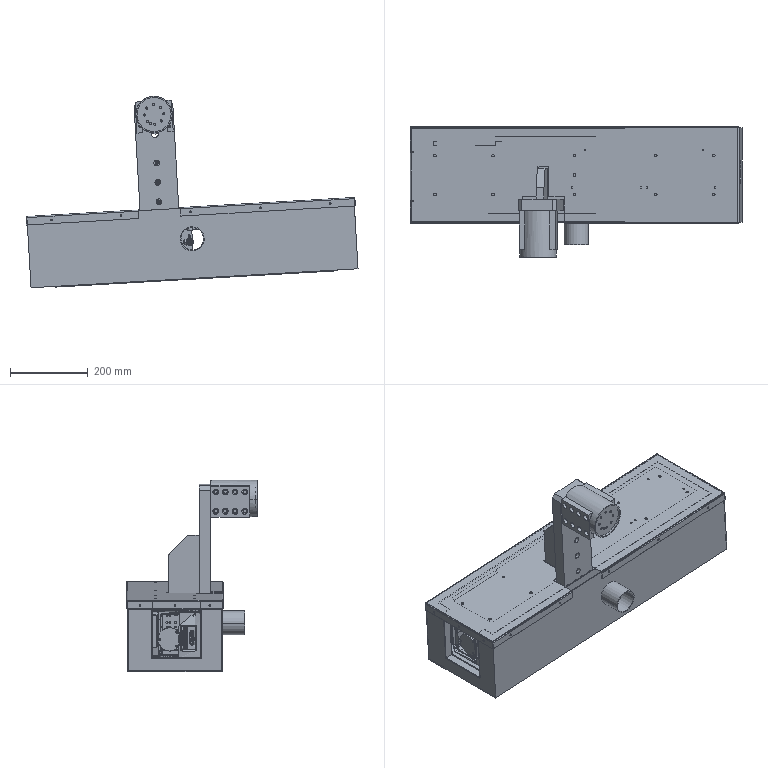Part | NX | features BREP 34 | 36 solids | 2839 faces | box 855.547 x 337 x 493.425 mm | volume 3563718 mm3 | cylinder 1301 | plane 1146 | cone 204 | spline 127 | torus 37 | sphere 24 | commonest cylinder face diameters 6 x193 0.7 x96 6.8 x66 15 x60 5 x50 5.5 x50